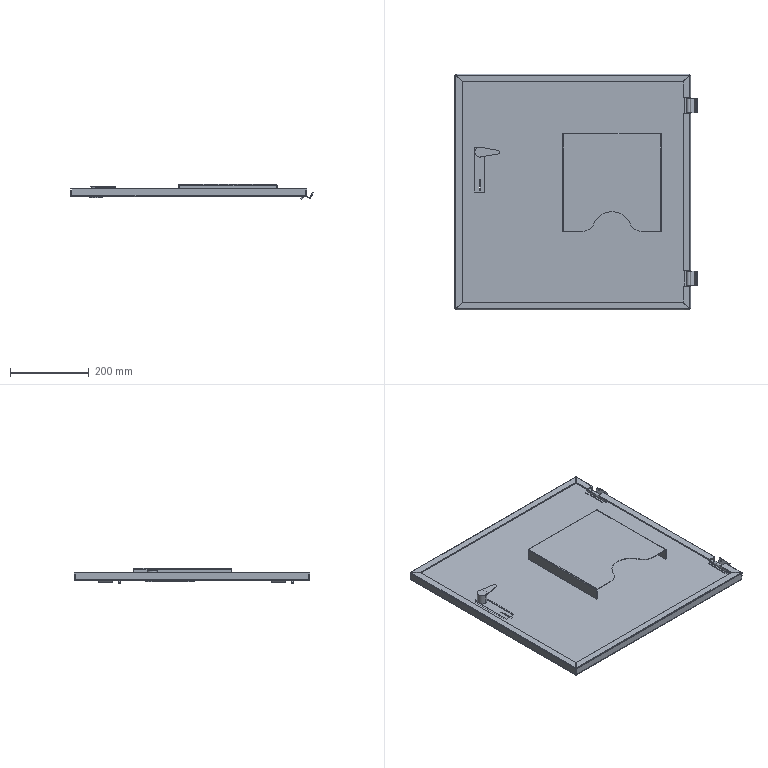Part | SolidWorks | features LocalLPattern 1, ReferencePattern 1 | 9 solids | 284 faces | box 616.798 x 600 x 38.851 mm | volume 818238 mm3 | plane 189 | cylinder 75 | spline 20 | commonest cylinder face diameters 5 x18 1.473 x15 4.473 x15 3.3 x8 9 x6 34 x3